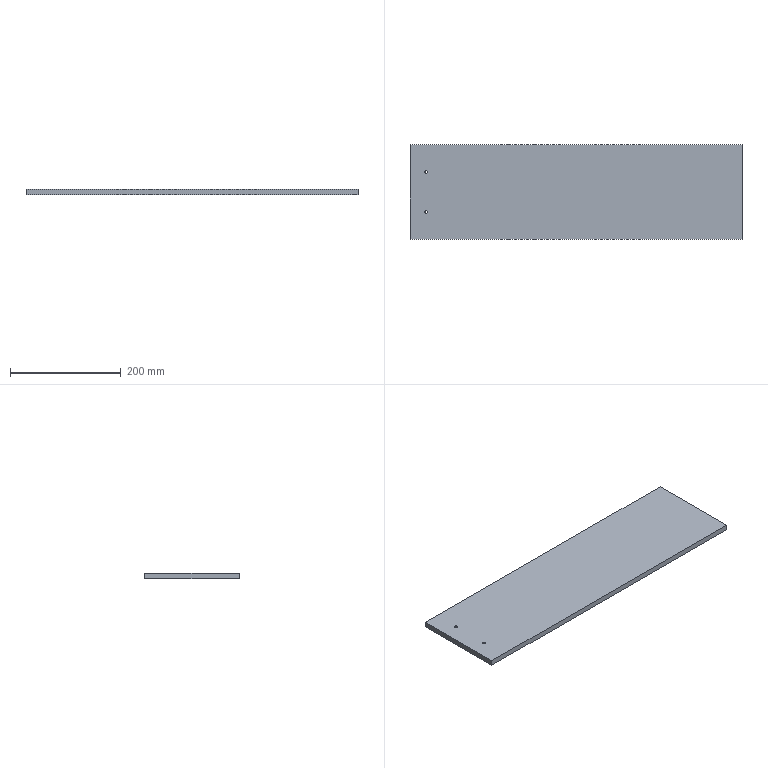Part | SolidWorks | features Extrusion 1, HoleWzd 1 | 1 solid | 10 faces | box 600 x 170 x 10 mm | volume 1019607 mm3 | plane 6 | cylinder 4 | commonest cylinder face diameters 5 x4
STEP:
#1=CARTESIAN_POINT('',(-273.25,36.25,10.));
#2=VERTEX_POINT('',#1);
#3=CARTESIAN_POINT('',(-268.25,36.25,10.));
#4=VERTEX_POINT('',#3);
#5=CARTESIAN_POINT('',(-270.75,36.25,10.));
#6=DIRECTION('',(0.,0.,1.));
#7=DIRECTION('',(1.,0.,0.));
#8=AXIS2_PLACEMENT_3D('',#5,#6,#7);
#9=CIRCLE('',#8,2.5);
#10=EDGE_CURVE('',#2,#4,#9,.T.);
#11=ORIENTED_EDGE('',*,*,#10,.T.);
#12=CARTESIAN_POINT('',(-268.25,36.25,0.));
#13=VERTEX_POINT('',#12);
#14=CARTESIAN_POINT('',(-268.25,36.25,0.));
#15=DIRECTION('',(0.,0.,-1.));
#16=VECTOR('',#15,1000.);
#17=LINE('',#14,#16);
#18=EDGE_CURVE('',#4,#13,#17,.T.);
#19=ORIENTED_EDGE('',*,*,#18,.T.);
#20=CARTESIAN_POINT('',(-273.25,36.25,0.));
#21=VERTEX_POINT('',#20);
#22=CARTESIAN_POINT('',(-270.75,36.25,0.));
#23=DIRECTION('',(0.,0.,-1.));
#24=DIRECTION('',(-1.,0.,0.));
#25=AXIS2_PLACEMENT_3D('',#22,#23,#24);
#26=CIRCLE('',#25,2.5);
#27=EDGE_CURVE('',#13,#21,#26,.T.);
#28=ORIENTED_EDGE('',*,*,#27,.T.);
#29=CARTESIAN_POINT('',(-273.25,36.25,0.));
#30=DIRECTION('',(0.,0.,-1.));
#31=VECTOR('',#30,1000.);
#32=LINE('',#29,#31);
#33=EDGE_CURVE('',#2,#21,#32,.T.);
#34=ORIENTED_EDGE('',*,*,#33,.F.);
#35=EDGE_LOOP('',(#11,#19,#28,#34));
#36=FACE_OUTER_BOUND('',#35,.T.);
#37=CARTESIAN_POINT('',(-270.75,36.25,0.));
#38=DIRECTION('',(0.,0.,-1.));
#39=DIRECTION('',(-1.,0.,0.));
#40=AXIS2_PLACEMENT_3D('',#37,#38,#39);
#41=CYLINDRICAL_SURFACE('',#40,2.5);
#42=ADVANCED_FACE('',(#36),#41,.F.);
#43=CARTESIAN_POINT('',(-273.25,-36.25,10.));
#44=VERTEX_POINT('',#43);
#45=CARTESIAN_POINT('',(-268.25,-36.25,10.));
#46=VERTEX_POINT('',#45);
#47=CARTESIAN_POINT('',(-270.75,-36.25,10.));
#48=DIRECTION('',(0.,0.,1.));
#49=DIRECTION('',(1.,0.,0.));
#50=AXIS2_PLACEMENT_3D('',#47,#48,#49);
#51=CIRCLE('',#50,2.5);
#52=EDGE_CURVE('',#44,#46,#51,.T.);
#53=ORIENTED_EDGE('',*,*,#52,.T.);
#54=CARTESIAN_POINT('',(-268.25,-36.25,0.));
#55=VERTEX_POINT('',#54);
#56=CARTESIAN_POINT('',(-268.25,-36.25,0.));
#57=DIRECTION('',(0.,0.,-1.));
#58=VECTOR('',#57,1000.);
#59=LINE('',#56,#58);
#60=EDGE_CURVE('',#46,#55,#59,.T.);
#61=ORIENTED_EDGE('',*,*,#60,.T.);
#62=CARTESIAN_POINT('',(-273.25,-36.25,0.));
#63=VERTEX_POINT('',#62);
#64=CARTESIAN_POINT('',(-270.75,-36.25,0.));
#65=DIRECTION('',(0.,0.,-1.));
#66=DIRECTION('',(-1.,0.,0.));
#67=AXIS2_PLACEMENT_3D('',#64,#65,#66);
#68=CIRCLE('',#67,2.5);
#69=EDGE_CURVE('',#55,#63,#68,.T.);
#70=ORIENTED_EDGE('',*,*,#69,.T.);
#71=CARTESIAN_POINT('',(-273.25,-36.25,0.));
#72=DIRECTION('',(0.,0.,-1.));
#73=VECTOR('',#72,1000.);
#74=LINE('',#71,#73);
#75=EDGE_CURVE('',#44,#63,#74,.T.);
#76=ORIENTED_EDGE('',*,*,#75,.F.);
#77=EDGE_LOOP('',(#53,#61,#70,#76));
#78=FACE_OUTER_BOUND('',#77,.T.);
#79=CARTESIAN_POINT('',(-270.75,-36.25,0.));
#80=DIRECTION('',(0.,0.,-1.));
#81=DIRECTION('',(-1.,0.,0.));
#82=AXIS2_PLACEMENT_3D('',#79,#80,#81);
#83=CYLINDRICAL_SURFACE('',#82,2.5);
#84=ADVANCED_FACE('',(#78),#83,.F.);
#85=CARTESIAN_POINT('',(300.,-85.,0.));
#86=VERTEX_POINT('',#85);
#87=CARTESIAN_POINT('',(300.,85.,0.));
#88=VERTEX_POINT('',#87);
#89=CARTESIAN_POINT('',(300.,85.,0.));
#90=DIRECTION('',(0.,1.,0.));
#91=VECTOR('',#90,1000.);
#92=LINE('',#89,#91);
#93=EDGE_CURVE('',#86,#88,#92,.T.);
#94=ORIENTED_EDGE('',*,*,#93,.T.);
#95=CARTESIAN_POINT('',(300.,85.,10.));
#96=VERTEX_POINT('',#95);
#97=CARTESIAN_POINT('',(300.,85.,10.));
#98=DIRECTION('',(0.,0.,-1.));
#99=VECTOR('',#98,1000.);
#100=LINE('',#97,#99);
#101=EDGE_CURVE('',#96,#88,#100,.T.);
#102=ORIENTED_EDGE('',*,*,#101,.F.);
#103=CARTESIAN_POINT('',(300.,-85.,10.));
#104=VERTEX_POINT('',#103);
#105=CARTESIAN_POINT('',(300.,85.,10.));
#106=DIRECTION('',(0.,1.,0.));
#107=VECTOR('',#106,1000.);
#108=LINE('',#105,#107);
#109=EDGE_CURVE('',#104,#96,#108,.T.);
#110=ORIENTED_EDGE('',*,*,#109,.F.);
#111=CARTESIAN_POINT('',(300.,-85.,10.));
#112=DIRECTION('',(0.,0.,-1.));
#113=VECTOR('',#112,1000.);
#114=LINE('',#111,#113);
#115=EDGE_CURVE('',#104,#86,#114,.T.);
#116=ORIENTED_EDGE('',*,*,#115,.T.);
#117=EDGE_LOOP('',(#94,#102,#110,#116));
#118=FACE_OUTER_BOUND('',#117,.T.);
#119=CARTESIAN_POINT('',(300.,85.,10.));
#120=DIRECTION('',(-1.,0.,0.));
#121=DIRECTION('',(0.,0.,1.));
#122=AXIS2_PLACEMENT_3D('',#119,#120,#121);
#123=PLANE('',#122);
#124=ADVANCED_FACE('',(#118),#123,.F.);
#125=CARTESIAN_POINT('',(-300.,85.,0.));
#126=VERTEX_POINT('',#125);
#127=CARTESIAN_POINT('',(-300.,85.,0.));
#128=DIRECTION('',(-1.,0.,0.));
#129=VECTOR('',#128,1000.);
#130=LINE('',#127,#129);
#131=EDGE_CURVE('',#88,#126,#130,.T.);
#132=ORIENTED_EDGE('',*,*,#131,.T.);
#133=CARTESIAN_POINT('',(-300.,85.,10.));
#134=VERTEX_POINT('',#133);
#135=CARTESIAN_POINT('',(-300.,85.,10.));
#136=DIRECTION('',(0.,0.,-1.));
#137=VECTOR('',#136,1000.);
#138=LINE('',#135,#137);
#139=EDGE_CURVE('',#134,#126,#138,.T.);
#140=ORIENTED_EDGE('',*,*,#139,.F.);
#141=CARTESIAN_POINT('',(-300.,85.,10.));
#142=DIRECTION('',(-1.,0.,0.));
#143=VECTOR('',#142,1000.);
#144=LINE('',#141,#143);
#145=EDGE_CURVE('',#96,#134,#144,.T.);
#146=ORIENTED_EDGE('',*,*,#145,.F.);
#147=ORIENTED_EDGE('',*,*,#101,.T.);
#148=EDGE_LOOP('',(#132,#140,#146,#147));
#149=FACE_OUTER_BOUND('',#148,.T.);
#150=CARTESIAN_POINT('',(-300.,85.,10.));
#151=DIRECTION('',(0.,-1.,0.));
#152=DIRECTION('',(0.,0.,-1.));
#153=AXIS2_PLACEMENT_3D('',#150,#151,#152);
#154=PLANE('',#153);
#155=ADVANCED_FACE('',(#149),#154,.F.);
#156=CARTESIAN_POINT('',(-300.,-85.,0.));
#157=VERTEX_POINT('',#156);
#158=CARTESIAN_POINT('',(-300.,85.,0.));
#159=DIRECTION('',(0.,-1.,0.));
#160=VECTOR('',#159,1000.);
#161=LINE('',#158,#160);
#162=EDGE_CURVE('',#126,#157,#161,.T.);
#163=ORIENTED_EDGE('',*,*,#162,.T.);
#164=CARTESIAN_POINT('',(-300.,-85.,10.));
#165=VERTEX_POINT('',#164);
#166=CARTESIAN_POINT('',(-300.,-85.,10.));
#167=DIRECTION('',(0.,0.,-1.));
#168=VECTOR('',#167,1000.);
#169=LINE('',#166,#168);
#170=EDGE_CURVE('',#165,#157,#169,.T.);
#171=ORIENTED_EDGE('',*,*,#170,.F.);
#172=CARTESIAN_POINT('',(-300.,85.,10.));
#173=DIRECTION('',(0.,-1.,0.));
#174=VECTOR('',#173,1000.);
#175=LINE('',#172,#174);
#176=EDGE_CURVE('',#134,#165,#175,.T.);
#177=ORIENTED_EDGE('',*,*,#176,.F.);
#178=ORIENTED_EDGE('',*,*,#139,.T.);
#179=EDGE_LOOP('',(#163,#171,#177,#178));
#180=FACE_OUTER_BOUND('',#179,.T.);
#181=CARTESIAN_POINT('',(-300.,85.,10.));
#182=DIRECTION('',(1.,0.,0.));
#183=DIRECTION('',(0.,1.,0.));
#184=AXIS2_PLACEMENT_3D('',#181,#182,#183);
#185=PLANE('',#184);
#186=ADVANCED_FACE('',(#180),#185,.F.);
#187=CARTESIAN_POINT('',(-300.,-85.,0.));
#188=DIRECTION('',(1.,0.,0.));
#189=VECTOR('',#188,1000.);
#190=LINE('',#187,#189);
#191=EDGE_CURVE('',#157,#86,#190,.T.);
#192=ORIENTED_EDGE('',*,*,#191,.T.);
#193=ORIENTED_EDGE('',*,*,#115,.F.);
#194=CARTESIAN_POINT('',(-300.,-85.,10.));
#195=DIRECTION('',(1.,0.,0.));
#196=VECTOR('',#195,1000.);
#197=LINE('',#194,#196);
#198=EDGE_CURVE('',#165,#104,#197,.T.);
#199=ORIENTED_EDGE('',*,*,#198,.F.);
#200=ORIENTED_EDGE('',*,*,#170,.T.);
#201=EDGE_LOOP('',(#192,#193,#199,#200));
#202=FACE_OUTER_BOUND('',#201,.T.);
#203=CARTESIAN_POINT('',(-300.,-85.,10.));
#204=DIRECTION('',(0.,1.,0.));
#205=DIRECTION('',(0.,0.,1.));
#206=AXIS2_PLACEMENT_3D('',#203,#204,#205);
#207=PLANE('',#206);
#208=ADVANCED_FACE('',(#202),#207,.F.);
#209=ORIENTED_EDGE('',*,*,#10,.F.);
#210=CARTESIAN_POINT('',(-270.75,36.25,10.));
#211=DIRECTION('',(0.,0.,1.));
#212=DIRECTION('',(1.,0.,0.));
#213=AXIS2_PLACEMENT_3D('',#210,#211,#212);
#214=CIRCLE('',#213,2.5);
#215=EDGE_CURVE('',#4,#2,#214,.T.);
#216=ORIENTED_EDGE('',*,*,#215,.F.);
#217=EDGE_LOOP('',(#209,#216));
#218=FACE_BOUND('',#217,.T.);
#219=ORIENTED_EDGE('',*,*,#52,.F.);
#220=CARTESIAN_POINT('',(-270.75,-36.25,10.));
#221=DIRECTION('',(0.,0.,1.));
#222=DIRECTION('',(1.,0.,0.));
#223=AXIS2_PLACEMENT_3D('',#220,#221,#222);
#224=CIRCLE('',#223,2.5);
#225=EDGE_CURVE('',#46,#44,#224,.T.);
#226=ORIENTED_EDGE('',*,*,#225,.F.);
#227=EDGE_LOOP('',(#219,#226));
#228=FACE_BOUND('',#227,.T.);
#229=ORIENTED_EDGE('',*,*,#109,.T.);
#230=ORIENTED_EDGE('',*,*,#145,.T.);
#231=ORIENTED_EDGE('',*,*,#176,.T.);
#232=ORIENTED_EDGE('',*,*,#198,.T.);
#233=EDGE_LOOP('',(#229,#230,#231,#232));
#234=FACE_OUTER_BOUND('',#233,.T.);
#235=CARTESIAN_POINT('',(0.,0.,10.));
#236=DIRECTION('',(0.,0.,1.));
#237=DIRECTION('',(1.,0.,0.));
#238=AXIS2_PLACEMENT_3D('',#235,#236,#237);
#239=PLANE('',#238);
#240=ADVANCED_FACE('',(#218,#228,#234),#239,.T.);
#241=CARTESIAN_POINT('',(-270.75,36.25,0.));
#242=DIRECTION('',(0.,0.,-1.));
#243=DIRECTION('',(-1.,0.,0.));
#244=AXIS2_PLACEMENT_3D('',#241,#242,#243);
#245=CIRCLE('',#244,2.5);
#246=EDGE_CURVE('',#21,#13,#245,.T.);
#247=ORIENTED_EDGE('',*,*,#246,.F.);
#248=ORIENTED_EDGE('',*,*,#27,.F.);
#249=EDGE_LOOP('',(#247,#248));
#250=FACE_BOUND('',#249,.T.);
#251=CARTESIAN_POINT('',(-270.75,-36.25,0.));
#252=DIRECTION('',(0.,0.,-1.));
#253=DIRECTION('',(-1.,0.,0.));
#254=AXIS2_PLACEMENT_3D('',#251,#252,#253);
#255=CIRCLE('',#254,2.5);
#256=EDGE_CURVE('',#63,#55,#255,.T.);
#257=ORIENTED_EDGE('',*,*,#256,.F.);
#258=ORIENTED_EDGE('',*,*,#69,.F.);
#259=EDGE_LOOP('',(#257,#258));
#260=FACE_BOUND('',#259,.T.);
#261=ORIENTED_EDGE('',*,*,#93,.F.);
#262=ORIENTED_EDGE('',*,*,#191,.F.);
#263=ORIENTED_EDGE('',*,*,#162,.F.);
#264=ORIENTED_EDGE('',*,*,#131,.F.);
#265=EDGE_LOOP('',(#261,#262,#263,#264));
#266=FACE_OUTER_BOUND('',#265,.T.);
#267=CARTESIAN_POINT('',(0.,0.,0.));
#268=DIRECTION('',(0.,0.,1.));
#269=DIRECTION('',(1.,0.,0.));
#270=AXIS2_PLACEMENT_3D('',#267,#268,#269);
#271=PLANE('',#270);
#272=ADVANCED_FACE('',(#250,#260,#266),#271,.F.);
#273=ORIENTED_EDGE('',*,*,#60,.F.);
#274=ORIENTED_EDGE('',*,*,#225,.T.);
#275=ORIENTED_EDGE('',*,*,#75,.T.);
#276=ORIENTED_EDGE('',*,*,#256,.T.);
#277=EDGE_LOOP('',(#273,#274,#275,#276));
#278=FACE_OUTER_BOUND('',#277,.T.);
#279=CARTESIAN_POINT('',(-270.75,-36.25,0.));
#280=DIRECTION('',(0.,0.,-1.));
#281=DIRECTION('',(-1.,0.,0.));
#282=AXIS2_PLACEMENT_3D('',#279,#280,#281);
#283=CYLINDRICAL_SURFACE('',#282,2.5);
#284=ADVANCED_FACE('',(#278),#283,.F.);
#285=ORIENTED_EDGE('',*,*,#18,.F.);
#286=ORIENTED_EDGE('',*,*,#215,.T.);
#287=ORIENTED_EDGE('',*,*,#33,.T.);
#288=ORIENTED_EDGE('',*,*,#246,.T.);
#289=EDGE_LOOP('',(#285,#286,#287,#288));
#290=FACE_OUTER_BOUND('',#289,.T.);
#291=CARTESIAN_POINT('',(-270.75,36.25,0.));
#292=DIRECTION('',(0.,0.,-1.));
#293=DIRECTION('',(-1.,0.,0.));
#294=AXIS2_PLACEMENT_3D('',#291,#292,#293);
#295=CYLINDRICAL_SURFACE('',#294,2.5);
#296=ADVANCED_FACE('',(#290),#295,.F.);
#297=CLOSED_SHELL('',(#42,#84,#124,#155,#186,#208,#240,#272,#284,#296));
#298=MANIFOLD_SOLID_BREP('',#297);
#299=CARTESIAN_POINT('',(0.,0.,0.));
#300=DIRECTION('',(0.,0.,1.));
#301=DIRECTION('',(1.,0.,0.));
#302=AXIS2_PLACEMENT_3D('',#299,#300,#301);
#303=(LENGTH_UNIT()NAMED_UNIT(*)SI_UNIT(.MILLI.,.METRE.));
#304=UNCERTAINTY_MEASURE_WITH_UNIT(LENGTH_MEASURE(0.00001),#303,'','');
#305=(NAMED_UNIT(*)PLANE_ANGLE_UNIT()SI_UNIT($,.RADIAN.));
#306=(NAMED_UNIT(*)SI_UNIT($,.STERADIAN.)SOLID_ANGLE_UNIT());
#307=(GEOMETRIC_REPRESENTATION_CONTEXT(3)GLOBAL_UNCERTAINTY_ASSIGNED_CONTEXT((#304))GLOBAL_UNIT_ASSIGNED_CONTEXT((#303,#305,#306))REPRESENTATION_CONTEXT('',''));
#308=ADVANCED_BREP_SHAPE_REPRESENTATION('',(#298,#302),#307);